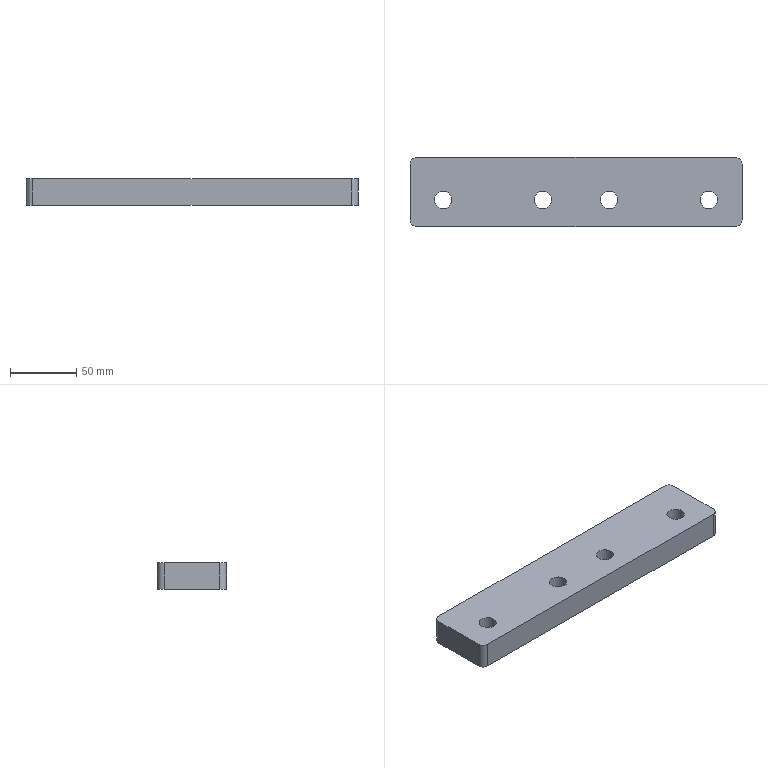Part | NX | features MAIN_BODY 2 | 1 solid | 14 faces | box 250 x 52 x 20 mm | volume 248952 mm3 | cylinder 8 | plane 6 | commonest cylinder face diameters 10 x4 13 x4
STEP:
#1=CARTESIAN_POINT('',(245.,837.,-175.));
#2=VERTEX_POINT('',#1);
#3=CARTESIAN_POINT('',(245.,795.,-175.));
#4=VERTEX_POINT('',#3);
#5=CARTESIAN_POINT('',(245.,842.,-175.));
#6=DIRECTION('',(0.,-1.,0.));
#7=VECTOR('',#6,1000.);
#8=LINE('',#5,#7);
#9=EDGE_CURVE('',#2,#4,#8,.T.);
#10=ORIENTED_EDGE('',*,*,#9,.F.);
#11=CARTESIAN_POINT('',(245.,837.,-195.));
#12=VERTEX_POINT('',#11);
#13=CARTESIAN_POINT('',(245.,837.,-195.));
#14=DIRECTION('',(0.,0.,1.));
#15=VECTOR('',#14,1000.);
#16=LINE('',#13,#15);
#17=EDGE_CURVE('',#2,#12,#16,.F.);
#18=ORIENTED_EDGE('',*,*,#17,.T.);
#19=CARTESIAN_POINT('',(245.,795.,-195.));
#20=VERTEX_POINT('',#19);
#21=CARTESIAN_POINT('',(245.,842.,-195.));
#22=DIRECTION('',(0.,-1.,0.));
#23=VECTOR('',#22,1000.);
#24=LINE('',#21,#23);
#25=EDGE_CURVE('',#12,#20,#24,.T.);
#26=ORIENTED_EDGE('',*,*,#25,.T.);
#27=CARTESIAN_POINT('',(245.,795.,-195.));
#28=DIRECTION('',(0.,0.,1.));
#29=VECTOR('',#28,1000.);
#30=LINE('',#27,#29);
#31=EDGE_CURVE('',#20,#4,#30,.T.);
#32=ORIENTED_EDGE('',*,*,#31,.T.);
#33=EDGE_LOOP('',(#10,#18,#26,#32));
#34=FACE_BOUND('',#33,.T.);
#35=CARTESIAN_POINT('',(245.,842.,-195.));
#36=DIRECTION('',(-1.,0.,0.));
#37=DIRECTION('',(0.,1.,0.));
#38=AXIS2_PLACEMENT_3D('',#35,#36,#37);
#39=PLANE('',#38);
#40=ADVANCED_FACE('',(#34),#39,.T.);
#41=CARTESIAN_POINT('',(250.,790.,-175.));
#42=VERTEX_POINT('',#41);
#43=CARTESIAN_POINT('',(490.,790.,-175.));
#44=VERTEX_POINT('',#43);
#45=CARTESIAN_POINT('',(245.,790.,-175.));
#46=DIRECTION('',(1.,0.,0.));
#47=VECTOR('',#46,1000.);
#48=LINE('',#45,#47);
#49=EDGE_CURVE('',#42,#44,#48,.T.);
#50=ORIENTED_EDGE('',*,*,#49,.F.);
#51=CARTESIAN_POINT('',(250.,790.,-195.));
#52=VERTEX_POINT('',#51);
#53=CARTESIAN_POINT('',(250.,790.,-195.));
#54=DIRECTION('',(0.,0.,1.));
#55=VECTOR('',#54,1000.);
#56=LINE('',#53,#55);
#57=EDGE_CURVE('',#42,#52,#56,.F.);
#58=ORIENTED_EDGE('',*,*,#57,.T.);
#59=CARTESIAN_POINT('',(490.,790.,-195.));
#60=VERTEX_POINT('',#59);
#61=CARTESIAN_POINT('',(245.,790.,-195.));
#62=DIRECTION('',(1.,0.,0.));
#63=VECTOR('',#62,1000.);
#64=LINE('',#61,#63);
#65=EDGE_CURVE('',#52,#60,#64,.T.);
#66=ORIENTED_EDGE('',*,*,#65,.T.);
#67=CARTESIAN_POINT('',(490.,790.,-195.));
#68=DIRECTION('',(0.,0.,1.));
#69=VECTOR('',#68,1000.);
#70=LINE('',#67,#69);
#71=EDGE_CURVE('',#60,#44,#70,.T.);
#72=ORIENTED_EDGE('',*,*,#71,.T.);
#73=EDGE_LOOP('',(#50,#58,#66,#72));
#74=FACE_BOUND('',#73,.T.);
#75=CARTESIAN_POINT('',(245.,790.,-195.));
#76=DIRECTION('',(0.,-1.,0.));
#77=DIRECTION('',(-1.,0.,0.));
#78=AXIS2_PLACEMENT_3D('',#75,#76,#77);
#79=PLANE('',#78);
#80=ADVANCED_FACE('',(#74),#79,.T.);
#81=CARTESIAN_POINT('',(490.,842.,-195.));
#82=VERTEX_POINT('',#81);
#83=CARTESIAN_POINT('',(250.,842.,-195.));
#84=VERTEX_POINT('',#83);
#85=CARTESIAN_POINT('',(370.,842.,-195.));
#86=DIRECTION('',(-1.,0.,0.));
#87=VECTOR('',#86,1000.);
#88=LINE('',#85,#87);
#89=EDGE_CURVE('',#82,#84,#88,.T.);
#90=ORIENTED_EDGE('',*,*,#89,.T.);
#91=CARTESIAN_POINT('',(250.,842.,-175.));
#92=VERTEX_POINT('',#91);
#93=CARTESIAN_POINT('',(250.,842.,-195.));
#94=DIRECTION('',(0.,0.,1.));
#95=VECTOR('',#94,1000.);
#96=LINE('',#93,#95);
#97=EDGE_CURVE('',#84,#92,#96,.T.);
#98=ORIENTED_EDGE('',*,*,#97,.T.);
#99=CARTESIAN_POINT('',(490.,842.,-175.));
#100=VERTEX_POINT('',#99);
#101=CARTESIAN_POINT('',(370.,842.,-175.));
#102=DIRECTION('',(-1.,0.,0.));
#103=VECTOR('',#102,1000.);
#104=LINE('',#101,#103);
#105=EDGE_CURVE('',#100,#92,#104,.T.);
#106=ORIENTED_EDGE('',*,*,#105,.F.);
#107=CARTESIAN_POINT('',(490.,842.,-195.));
#108=DIRECTION('',(0.,0.,1.));
#109=VECTOR('',#108,1000.);
#110=LINE('',#107,#109);
#111=EDGE_CURVE('',#100,#82,#110,.F.);
#112=ORIENTED_EDGE('',*,*,#111,.T.);
#113=EDGE_LOOP('',(#90,#98,#106,#112));
#114=FACE_BOUND('',#113,.T.);
#115=CARTESIAN_POINT('',(370.,842.,-195.));
#116=DIRECTION('',(0.,1.,0.));
#117=DIRECTION('',(0.,0.,-1.));
#118=AXIS2_PLACEMENT_3D('',#115,#116,#117);
#119=PLANE('',#118);
#120=ADVANCED_FACE('',(#114),#119,.T.);
#121=CARTESIAN_POINT('',(351.5,810.,-195.));
#122=VERTEX_POINT('',#121);
#123=CARTESIAN_POINT('',(345.,810.,-195.));
#124=DIRECTION('',(0.,0.,1.));
#125=DIRECTION('',(1.,0.,0.));
#126=AXIS2_PLACEMENT_3D('',#123,#124,#125);
#127=CIRCLE('',#126,6.5);
#128=EDGE_CURVE('',#122,#122,#127,.T.);
#129=ORIENTED_EDGE('',*,*,#128,.T.);
#130=EDGE_LOOP('',(#129));
#131=FACE_BOUND('',#130,.T.);
#132=CARTESIAN_POINT('',(276.5,810.,-195.));
#133=VERTEX_POINT('',#132);
#134=CARTESIAN_POINT('',(270.,810.,-195.));
#135=DIRECTION('',(0.,0.,1.));
#136=DIRECTION('',(1.,0.,0.));
#137=AXIS2_PLACEMENT_3D('',#134,#135,#136);
#138=CIRCLE('',#137,6.5);
#139=EDGE_CURVE('',#133,#133,#138,.T.);
#140=ORIENTED_EDGE('',*,*,#139,.T.);
#141=EDGE_LOOP('',(#140));
#142=FACE_BOUND('',#141,.T.);
#143=ORIENTED_EDGE('',*,*,#25,.F.);
#144=CARTESIAN_POINT('',(250.,837.,-195.));
#145=DIRECTION('',(0.,0.,1.));
#146=DIRECTION('',(1.,0.,0.));
#147=AXIS2_PLACEMENT_3D('',#144,#145,#146);
#148=CIRCLE('',#147,5.);
#149=EDGE_CURVE('',#12,#84,#148,.F.);
#150=ORIENTED_EDGE('',*,*,#149,.T.);
#151=ORIENTED_EDGE('',*,*,#89,.F.);
#152=CARTESIAN_POINT('',(495.,837.,-195.));
#153=VERTEX_POINT('',#152);
#154=CARTESIAN_POINT('',(490.,837.,-195.));
#155=DIRECTION('',(0.,0.,1.));
#156=DIRECTION('',(1.,0.,0.));
#157=AXIS2_PLACEMENT_3D('',#154,#155,#156);
#158=CIRCLE('',#157,5.);
#159=EDGE_CURVE('',#82,#153,#158,.F.);
#160=ORIENTED_EDGE('',*,*,#159,.T.);
#161=CARTESIAN_POINT('',(495.,795.,-195.));
#162=VERTEX_POINT('',#161);
#163=CARTESIAN_POINT('',(495.,842.,-195.));
#164=DIRECTION('',(0.,-1.,0.));
#165=VECTOR('',#164,1000.);
#166=LINE('',#163,#165);
#167=EDGE_CURVE('',#153,#162,#166,.T.);
#168=ORIENTED_EDGE('',*,*,#167,.T.);
#169=CARTESIAN_POINT('',(490.,795.,-195.));
#170=DIRECTION('',(0.,0.,1.));
#171=DIRECTION('',(1.,0.,0.));
#172=AXIS2_PLACEMENT_3D('',#169,#170,#171);
#173=CIRCLE('',#172,5.);
#174=EDGE_CURVE('',#162,#60,#173,.F.);
#175=ORIENTED_EDGE('',*,*,#174,.T.);
#176=ORIENTED_EDGE('',*,*,#65,.F.);
#177=CARTESIAN_POINT('',(250.,795.,-195.));
#178=DIRECTION('',(0.,0.,1.));
#179=DIRECTION('',(1.,0.,0.));
#180=AXIS2_PLACEMENT_3D('',#177,#178,#179);
#181=CIRCLE('',#180,5.);
#182=EDGE_CURVE('',#52,#20,#181,.F.);
#183=ORIENTED_EDGE('',*,*,#182,.T.);
#184=EDGE_LOOP('',(#143,#150,#151,#160,#168,#175,#176,#183));
#185=FACE_BOUND('',#184,.T.);
#186=CARTESIAN_POINT('',(388.5,810.,-195.));
#187=VERTEX_POINT('',#186);
#188=CARTESIAN_POINT('',(395.,810.,-195.));
#189=DIRECTION('',(0.,0.,-1.));
#190=DIRECTION('',(-1.,0.,0.));
#191=AXIS2_PLACEMENT_3D('',#188,#189,#190);
#192=CIRCLE('',#191,6.5);
#193=EDGE_CURVE('',#187,#187,#192,.T.);
#194=ORIENTED_EDGE('',*,*,#193,.F.);
#195=EDGE_LOOP('',(#194));
#196=FACE_BOUND('',#195,.T.);
#197=CARTESIAN_POINT('',(463.5,810.,-195.));
#198=VERTEX_POINT('',#197);
#199=CARTESIAN_POINT('',(470.,810.,-195.));
#200=DIRECTION('',(0.,0.,-1.));
#201=DIRECTION('',(-1.,0.,0.));
#202=AXIS2_PLACEMENT_3D('',#199,#200,#201);
#203=CIRCLE('',#202,6.5);
#204=EDGE_CURVE('',#198,#198,#203,.T.);
#205=ORIENTED_EDGE('',*,*,#204,.F.);
#206=EDGE_LOOP('',(#205));
#207=FACE_BOUND('',#206,.T.);
#208=CARTESIAN_POINT('',(245.,790.,-195.));
#209=DIRECTION('',(0.,0.,1.));
#210=DIRECTION('',(1.,0.,0.));
#211=AXIS2_PLACEMENT_3D('',#208,#209,#210);
#212=PLANE('',#211);
#213=ADVANCED_FACE('',(#131,#142,#185,#196,#207),#212,.F.);
#214=CARTESIAN_POINT('',(351.5,810.,-175.));
#215=VERTEX_POINT('',#214);
#216=CARTESIAN_POINT('',(345.,810.,-175.));
#217=DIRECTION('',(0.,0.,1.));
#218=DIRECTION('',(1.,0.,0.));
#219=AXIS2_PLACEMENT_3D('',#216,#217,#218);
#220=CIRCLE('',#219,6.5);
#221=EDGE_CURVE('',#215,#215,#220,.T.);
#222=ORIENTED_EDGE('',*,*,#221,.F.);
#223=EDGE_LOOP('',(#222));
#224=FACE_BOUND('',#223,.T.);
#225=CARTESIAN_POINT('',(276.5,810.,-175.));
#226=VERTEX_POINT('',#225);
#227=CARTESIAN_POINT('',(270.,810.,-175.));
#228=DIRECTION('',(0.,0.,1.));
#229=DIRECTION('',(1.,0.,0.));
#230=AXIS2_PLACEMENT_3D('',#227,#228,#229);
#231=CIRCLE('',#230,6.5);
#232=EDGE_CURVE('',#226,#226,#231,.T.);
#233=ORIENTED_EDGE('',*,*,#232,.F.);
#234=EDGE_LOOP('',(#233));
#235=FACE_BOUND('',#234,.T.);
#236=ORIENTED_EDGE('',*,*,#105,.T.);
#237=CARTESIAN_POINT('',(250.,837.,-175.));
#238=DIRECTION('',(0.,0.,1.));
#239=DIRECTION('',(1.,0.,0.));
#240=AXIS2_PLACEMENT_3D('',#237,#238,#239);
#241=CIRCLE('',#240,5.);
#242=EDGE_CURVE('',#92,#2,#241,.T.);
#243=ORIENTED_EDGE('',*,*,#242,.T.);
#244=ORIENTED_EDGE('',*,*,#9,.T.);
#245=CARTESIAN_POINT('',(250.,795.,-175.));
#246=DIRECTION('',(0.,0.,1.));
#247=DIRECTION('',(1.,0.,0.));
#248=AXIS2_PLACEMENT_3D('',#245,#246,#247);
#249=CIRCLE('',#248,5.);
#250=EDGE_CURVE('',#4,#42,#249,.T.);
#251=ORIENTED_EDGE('',*,*,#250,.T.);
#252=ORIENTED_EDGE('',*,*,#49,.T.);
#253=CARTESIAN_POINT('',(495.,795.,-175.));
#254=VERTEX_POINT('',#253);
#255=CARTESIAN_POINT('',(490.,795.,-175.));
#256=DIRECTION('',(0.,0.,1.));
#257=DIRECTION('',(1.,0.,0.));
#258=AXIS2_PLACEMENT_3D('',#255,#256,#257);
#259=CIRCLE('',#258,5.);
#260=EDGE_CURVE('',#44,#254,#259,.T.);
#261=ORIENTED_EDGE('',*,*,#260,.T.);
#262=CARTESIAN_POINT('',(495.,837.,-175.));
#263=VERTEX_POINT('',#262);
#264=CARTESIAN_POINT('',(495.,842.,-175.));
#265=DIRECTION('',(0.,-1.,0.));
#266=VECTOR('',#265,1000.);
#267=LINE('',#264,#266);
#268=EDGE_CURVE('',#263,#254,#267,.T.);
#269=ORIENTED_EDGE('',*,*,#268,.F.);
#270=CARTESIAN_POINT('',(490.,837.,-175.));
#271=DIRECTION('',(0.,0.,1.));
#272=DIRECTION('',(1.,0.,0.));
#273=AXIS2_PLACEMENT_3D('',#270,#271,#272);
#274=CIRCLE('',#273,5.);
#275=EDGE_CURVE('',#263,#100,#274,.T.);
#276=ORIENTED_EDGE('',*,*,#275,.T.);
#277=EDGE_LOOP('',(#236,#243,#244,#251,#252,#261,#269,#276));
#278=FACE_BOUND('',#277,.T.);
#279=CARTESIAN_POINT('',(388.5,810.,-175.));
#280=VERTEX_POINT('',#279);
#281=CARTESIAN_POINT('',(395.,810.,-175.));
#282=DIRECTION('',(0.,0.,-1.));
#283=DIRECTION('',(-1.,0.,0.));
#284=AXIS2_PLACEMENT_3D('',#281,#282,#283);
#285=CIRCLE('',#284,6.5);
#286=EDGE_CURVE('',#280,#280,#285,.T.);
#287=ORIENTED_EDGE('',*,*,#286,.T.);
#288=EDGE_LOOP('',(#287));
#289=FACE_BOUND('',#288,.T.);
#290=CARTESIAN_POINT('',(463.5,810.,-175.));
#291=VERTEX_POINT('',#290);
#292=CARTESIAN_POINT('',(470.,810.,-175.));
#293=DIRECTION('',(0.,0.,-1.));
#294=DIRECTION('',(-1.,0.,0.));
#295=AXIS2_PLACEMENT_3D('',#292,#293,#294);
#296=CIRCLE('',#295,6.5);
#297=EDGE_CURVE('',#291,#291,#296,.T.);
#298=ORIENTED_EDGE('',*,*,#297,.T.);
#299=EDGE_LOOP('',(#298));
#300=FACE_BOUND('',#299,.T.);
#301=CARTESIAN_POINT('',(245.,790.,-175.));
#302=DIRECTION('',(0.,0.,1.));
#303=DIRECTION('',(1.,0.,0.));
#304=AXIS2_PLACEMENT_3D('',#301,#302,#303);
#305=PLANE('',#304);
#306=ADVANCED_FACE('',(#224,#235,#278,#289,#300),#305,.T.);
#307=ORIENTED_EDGE('',*,*,#232,.T.);
#308=EDGE_LOOP('',(#307));
#309=FACE_BOUND('',#308,.T.);
#310=ORIENTED_EDGE('',*,*,#139,.F.);
#311=EDGE_LOOP('',(#310));
#312=FACE_BOUND('',#311,.T.);
#313=CARTESIAN_POINT('',(270.,810.,-195.));
#314=DIRECTION('',(0.,0.,1.));
#315=DIRECTION('',(1.,0.,0.));
#316=AXIS2_PLACEMENT_3D('',#313,#314,#315);
#317=CYLINDRICAL_SURFACE('',#316,6.5);
#318=ADVANCED_FACE('',(#309,#312),#317,.F.);
#319=ORIENTED_EDGE('',*,*,#221,.T.);
#320=EDGE_LOOP('',(#319));
#321=FACE_BOUND('',#320,.T.);
#322=ORIENTED_EDGE('',*,*,#128,.F.);
#323=EDGE_LOOP('',(#322));
#324=FACE_BOUND('',#323,.T.);
#325=CARTESIAN_POINT('',(345.,810.,-195.));
#326=DIRECTION('',(0.,0.,1.));
#327=DIRECTION('',(1.,0.,0.));
#328=AXIS2_PLACEMENT_3D('',#325,#326,#327);
#329=CYLINDRICAL_SURFACE('',#328,6.5);
#330=ADVANCED_FACE('',(#321,#324),#329,.F.);
#331=ORIENTED_EDGE('',*,*,#167,.F.);
#332=CARTESIAN_POINT('',(495.,837.,-195.));
#333=DIRECTION('',(0.,0.,1.));
#334=VECTOR('',#333,1000.);
#335=LINE('',#332,#334);
#336=EDGE_CURVE('',#153,#263,#335,.T.);
#337=ORIENTED_EDGE('',*,*,#336,.T.);
#338=ORIENTED_EDGE('',*,*,#268,.T.);
#339=CARTESIAN_POINT('',(495.,795.,-195.));
#340=DIRECTION('',(0.,0.,1.));
#341=VECTOR('',#340,1000.);
#342=LINE('',#339,#341);
#343=EDGE_CURVE('',#254,#162,#342,.F.);
#344=ORIENTED_EDGE('',*,*,#343,.T.);
#345=EDGE_LOOP('',(#331,#337,#338,#344));
#346=FACE_BOUND('',#345,.T.);
#347=CARTESIAN_POINT('',(495.,842.,-195.));
#348=DIRECTION('',(1.,0.,0.));
#349=DIRECTION('',(0.,1.,0.));
#350=AXIS2_PLACEMENT_3D('',#347,#348,#349);
#351=PLANE('',#350);
#352=ADVANCED_FACE('',(#346),#351,.T.);
#353=ORIENTED_EDGE('',*,*,#297,.F.);
#354=EDGE_LOOP('',(#353));
#355=FACE_BOUND('',#354,.T.);
#356=ORIENTED_EDGE('',*,*,#204,.T.);
#357=EDGE_LOOP('',(#356));
#358=FACE_BOUND('',#357,.T.);
#359=CARTESIAN_POINT('',(470.,810.,-195.));
#360=DIRECTION('',(0.,0.,1.));
#361=DIRECTION('',(-1.,0.,0.));
#362=AXIS2_PLACEMENT_3D('',#359,#360,#361);
#363=CYLINDRICAL_SURFACE('',#362,6.5);
#364=ADVANCED_FACE('',(#355,#358),#363,.F.);
#365=ORIENTED_EDGE('',*,*,#286,.F.);
#366=EDGE_LOOP('',(#365));
#367=FACE_BOUND('',#366,.T.);
#368=ORIENTED_EDGE('',*,*,#193,.T.);
#369=EDGE_LOOP('',(#368));
#370=FACE_BOUND('',#369,.T.);
#371=CARTESIAN_POINT('',(395.,810.,-195.));
#372=DIRECTION('',(0.,0.,1.));
#373=DIRECTION('',(-1.,0.,0.));
#374=AXIS2_PLACEMENT_3D('',#371,#372,#373);
#375=CYLINDRICAL_SURFACE('',#374,6.5);
#376=ADVANCED_FACE('',(#367,#370),#375,.F.);
#377=ORIENTED_EDGE('',*,*,#149,.F.);
#378=ORIENTED_EDGE('',*,*,#17,.F.);
#379=ORIENTED_EDGE('',*,*,#242,.F.);
#380=ORIENTED_EDGE('',*,*,#97,.F.);
#381=EDGE_LOOP('',(#377,#378,#379,#380));
#382=FACE_BOUND('',#381,.T.);
#383=CARTESIAN_POINT('',(250.,837.,-195.));
#384=DIRECTION('',(0.,0.,1.));
#385=DIRECTION('',(1.,0.,0.));
#386=AXIS2_PLACEMENT_3D('',#383,#384,#385);
#387=CYLINDRICAL_SURFACE('',#386,5.);
#388=ADVANCED_FACE('',(#382),#387,.T.);
#389=ORIENTED_EDGE('',*,*,#182,.F.);
#390=ORIENTED_EDGE('',*,*,#57,.F.);
#391=ORIENTED_EDGE('',*,*,#250,.F.);
#392=ORIENTED_EDGE('',*,*,#31,.F.);
#393=EDGE_LOOP('',(#389,#390,#391,#392));
#394=FACE_BOUND('',#393,.T.);
#395=CARTESIAN_POINT('',(250.,795.,-195.));
#396=DIRECTION('',(0.,0.,1.));
#397=DIRECTION('',(1.,0.,0.));
#398=AXIS2_PLACEMENT_3D('',#395,#396,#397);
#399=CYLINDRICAL_SURFACE('',#398,5.);
#400=ADVANCED_FACE('',(#394),#399,.T.);
#401=ORIENTED_EDGE('',*,*,#159,.F.);
#402=ORIENTED_EDGE('',*,*,#111,.F.);
#403=ORIENTED_EDGE('',*,*,#275,.F.);
#404=ORIENTED_EDGE('',*,*,#336,.F.);
#405=EDGE_LOOP('',(#401,#402,#403,#404));
#406=FACE_BOUND('',#405,.T.);
#407=CARTESIAN_POINT('',(490.,837.,-195.));
#408=DIRECTION('',(0.,0.,1.));
#409=DIRECTION('',(1.,0.,0.));
#410=AXIS2_PLACEMENT_3D('',#407,#408,#409);
#411=CYLINDRICAL_SURFACE('',#410,5.);
#412=ADVANCED_FACE('',(#406),#411,.T.);
#413=ORIENTED_EDGE('',*,*,#174,.F.);
#414=ORIENTED_EDGE('',*,*,#343,.F.);
#415=ORIENTED_EDGE('',*,*,#260,.F.);
#416=ORIENTED_EDGE('',*,*,#71,.F.);
#417=EDGE_LOOP('',(#413,#414,#415,#416));
#418=FACE_BOUND('',#417,.T.);
#419=CARTESIAN_POINT('',(490.,795.,-195.));
#420=DIRECTION('',(0.,0.,1.));
#421=DIRECTION('',(1.,0.,0.));
#422=AXIS2_PLACEMENT_3D('',#419,#420,#421);
#423=CYLINDRICAL_SURFACE('',#422,5.);
#424=ADVANCED_FACE('',(#418),#423,.T.);
#425=CLOSED_SHELL('',(#40,#80,#120,#213,#306,#318,#330,#352,#364,#376,#388,#400,#412,#424));
#426=MANIFOLD_SOLID_BREP('',#425);
#427=(LENGTH_UNIT()NAMED_UNIT(*)SI_UNIT(.MILLI.,.METRE.));
#428=UNCERTAINTY_MEASURE_WITH_UNIT(LENGTH_MEASURE(0.00001),#427,'','');
#429=(NAMED_UNIT(*)PLANE_ANGLE_UNIT()SI_UNIT($,.RADIAN.));
#430=(NAMED_UNIT(*)SI_UNIT($,.STERADIAN.)SOLID_ANGLE_UNIT());
#431=(GEOMETRIC_REPRESENTATION_CONTEXT(3)GLOBAL_UNCERTAINTY_ASSIGNED_CONTEXT((#428))GLOBAL_UNIT_ASSIGNED_CONTEXT((#427,#429,#430))REPRESENTATION_CONTEXT('',''));
#432=ADVANCED_BREP_SHAPE_REPRESENTATION('',(#426),#431);